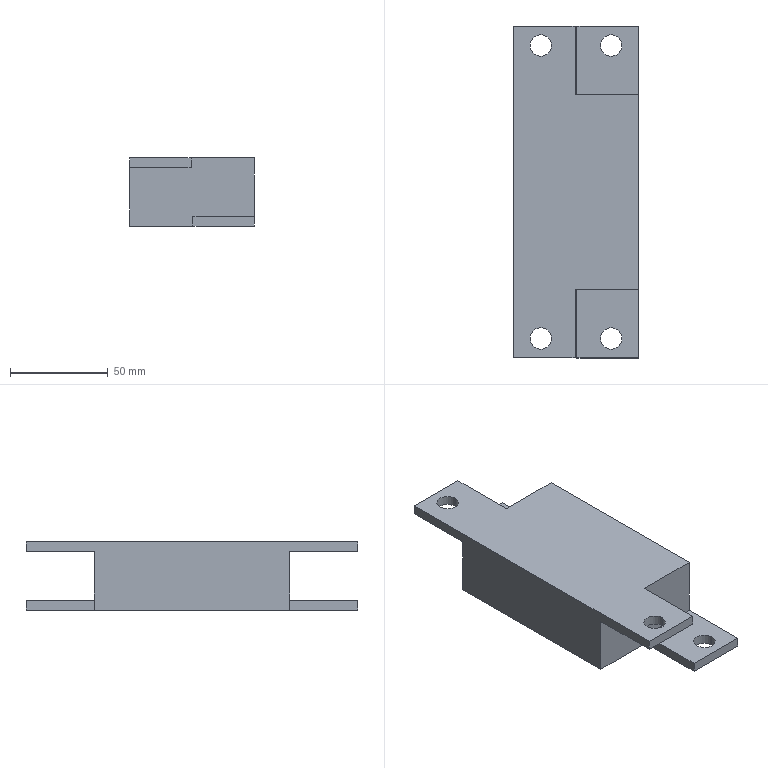Part | SolidWorks | features ICE 3, Extrusion 1 | 1 solid | 26 faces | box 64 x 170 x 35 mm | volume 244149 mm3 | plane 18 | cylinder 8 | commonest cylinder face diameters 11 x8
STEP:
#1=CARTESIAN_POINT('',(12.5,-75.,0.));
#2=VERTEX_POINT('',#1);
#3=CARTESIAN_POINT('',(23.5,-75.,0.));
#4=VERTEX_POINT('',#3);
#5=CARTESIAN_POINT('',(18.,-75.,0.));
#6=DIRECTION('',(0.,0.,1.));
#7=DIRECTION('',(-1.,0.,0.));
#8=AXIS2_PLACEMENT_3D('',#5,#6,#7);
#9=CIRCLE('',#8,5.5);
#10=EDGE_CURVE('',#2,#4,#9,.T.);
#11=ORIENTED_EDGE('',*,*,#10,.F.);
#12=CARTESIAN_POINT('',(12.5,-75.,5.));
#13=VERTEX_POINT('',#12);
#14=CARTESIAN_POINT('',(12.5,-75.,0.));
#15=DIRECTION('',(0.,0.,1.));
#16=VECTOR('',#15,1000.);
#17=LINE('',#14,#16);
#18=EDGE_CURVE('',#2,#13,#17,.T.);
#19=ORIENTED_EDGE('',*,*,#18,.T.);
#20=CARTESIAN_POINT('',(23.5,-75.,5.));
#21=VERTEX_POINT('',#20);
#22=CARTESIAN_POINT('',(18.,-75.,5.));
#23=DIRECTION('',(0.,0.,1.));
#24=DIRECTION('',(1.,0.,0.));
#25=AXIS2_PLACEMENT_3D('',#22,#23,#24);
#26=CIRCLE('',#25,5.5);
#27=EDGE_CURVE('',#13,#21,#26,.T.);
#28=ORIENTED_EDGE('',*,*,#27,.T.);
#29=CARTESIAN_POINT('',(23.5,-75.,0.));
#30=DIRECTION('',(0.,0.,1.));
#31=VECTOR('',#30,1000.);
#32=LINE('',#29,#31);
#33=EDGE_CURVE('',#4,#21,#32,.T.);
#34=ORIENTED_EDGE('',*,*,#33,.F.);
#35=EDGE_LOOP('',(#11,#19,#28,#34));
#36=FACE_OUTER_BOUND('',#35,.T.);
#37=CARTESIAN_POINT('',(18.,-75.,0.));
#38=DIRECTION('',(0.,0.,1.));
#39=DIRECTION('',(1.,0.,0.));
#40=AXIS2_PLACEMENT_3D('',#37,#38,#39);
#41=CYLINDRICAL_SURFACE('',#40,5.5);
#42=ADVANCED_FACE('',(#36),#41,.F.);
#43=CARTESIAN_POINT('',(12.5,75.,0.));
#44=VERTEX_POINT('',#43);
#45=CARTESIAN_POINT('',(23.5,75.,0.));
#46=VERTEX_POINT('',#45);
#47=CARTESIAN_POINT('',(18.,75.,0.));
#48=DIRECTION('',(0.,0.,1.));
#49=DIRECTION('',(1.,0.,0.));
#50=AXIS2_PLACEMENT_3D('',#47,#48,#49);
#51=CIRCLE('',#50,5.5);
#52=EDGE_CURVE('',#44,#46,#51,.T.);
#53=ORIENTED_EDGE('',*,*,#52,.F.);
#54=CARTESIAN_POINT('',(12.5,75.,5.));
#55=VERTEX_POINT('',#54);
#56=CARTESIAN_POINT('',(12.5,75.,0.));
#57=DIRECTION('',(0.,0.,1.));
#58=VECTOR('',#57,1000.);
#59=LINE('',#56,#58);
#60=EDGE_CURVE('',#44,#55,#59,.T.);
#61=ORIENTED_EDGE('',*,*,#60,.T.);
#62=CARTESIAN_POINT('',(23.5,75.,5.));
#63=VERTEX_POINT('',#62);
#64=CARTESIAN_POINT('',(18.,75.,5.));
#65=DIRECTION('',(0.,0.,-1.));
#66=DIRECTION('',(-1.,0.,0.));
#67=AXIS2_PLACEMENT_3D('',#64,#65,#66);
#68=CIRCLE('',#67,5.5);
#69=EDGE_CURVE('',#63,#55,#68,.T.);
#70=ORIENTED_EDGE('',*,*,#69,.F.);
#71=CARTESIAN_POINT('',(23.5,75.,0.));
#72=DIRECTION('',(0.,0.,1.));
#73=VECTOR('',#72,1000.);
#74=LINE('',#71,#73);
#75=EDGE_CURVE('',#46,#63,#74,.T.);
#76=ORIENTED_EDGE('',*,*,#75,.F.);
#77=EDGE_LOOP('',(#53,#61,#70,#76));
#78=FACE_OUTER_BOUND('',#77,.T.);
#79=CARTESIAN_POINT('',(18.,75.,0.));
#80=DIRECTION('',(0.,0.,1.));
#81=DIRECTION('',(1.,0.,0.));
#82=AXIS2_PLACEMENT_3D('',#79,#80,#81);
#83=CYLINDRICAL_SURFACE('',#82,5.5);
#84=ADVANCED_FACE('',(#78),#83,.F.);
#85=CARTESIAN_POINT('',(-23.5,75.,30.));
#86=VERTEX_POINT('',#85);
#87=CARTESIAN_POINT('',(-12.5,75.,30.));
#88=VERTEX_POINT('',#87);
#89=CARTESIAN_POINT('',(-18.,75.,30.));
#90=DIRECTION('',(0.,0.,1.));
#91=DIRECTION('',(1.,0.,0.));
#92=AXIS2_PLACEMENT_3D('',#89,#90,#91);
#93=CIRCLE('',#92,5.5);
#94=EDGE_CURVE('',#86,#88,#93,.T.);
#95=ORIENTED_EDGE('',*,*,#94,.F.);
#96=CARTESIAN_POINT('',(-23.5,75.,35.));
#97=VERTEX_POINT('',#96);
#98=CARTESIAN_POINT('',(-23.5,75.,0.));
#99=DIRECTION('',(0.,0.,1.));
#100=VECTOR('',#99,1000.);
#101=LINE('',#98,#100);
#102=EDGE_CURVE('',#86,#97,#101,.T.);
#103=ORIENTED_EDGE('',*,*,#102,.T.);
#104=CARTESIAN_POINT('',(-12.5,75.,35.));
#105=VERTEX_POINT('',#104);
#106=CARTESIAN_POINT('',(-18.,75.,35.));
#107=DIRECTION('',(0.,0.,1.));
#108=DIRECTION('',(1.,0.,0.));
#109=AXIS2_PLACEMENT_3D('',#106,#107,#108);
#110=CIRCLE('',#109,5.5);
#111=EDGE_CURVE('',#97,#105,#110,.T.);
#112=ORIENTED_EDGE('',*,*,#111,.T.);
#113=CARTESIAN_POINT('',(-12.5,75.,0.));
#114=DIRECTION('',(0.,0.,1.));
#115=VECTOR('',#114,1000.);
#116=LINE('',#113,#115);
#117=EDGE_CURVE('',#88,#105,#116,.T.);
#118=ORIENTED_EDGE('',*,*,#117,.F.);
#119=EDGE_LOOP('',(#95,#103,#112,#118));
#120=FACE_OUTER_BOUND('',#119,.T.);
#121=CARTESIAN_POINT('',(-18.,75.,0.));
#122=DIRECTION('',(0.,0.,1.));
#123=DIRECTION('',(1.,0.,0.));
#124=AXIS2_PLACEMENT_3D('',#121,#122,#123);
#125=CYLINDRICAL_SURFACE('',#124,5.5);
#126=ADVANCED_FACE('',(#120),#125,.F.);
#127=CARTESIAN_POINT('',(-12.5,-75.,30.));
#128=VERTEX_POINT('',#127);
#129=CARTESIAN_POINT('',(-23.5,-75.,30.));
#130=VERTEX_POINT('',#129);
#131=CARTESIAN_POINT('',(-18.,-75.,30.));
#132=DIRECTION('',(0.,0.,-1.));
#133=DIRECTION('',(-1.,0.,0.));
#134=AXIS2_PLACEMENT_3D('',#131,#132,#133);
#135=CIRCLE('',#134,5.5);
#136=EDGE_CURVE('',#128,#130,#135,.T.);
#137=ORIENTED_EDGE('',*,*,#136,.T.);
#138=CARTESIAN_POINT('',(-23.5,-75.,35.));
#139=VERTEX_POINT('',#138);
#140=CARTESIAN_POINT('',(-23.5,-75.,0.));
#141=DIRECTION('',(0.,0.,1.));
#142=VECTOR('',#141,1000.);
#143=LINE('',#140,#142);
#144=EDGE_CURVE('',#130,#139,#143,.T.);
#145=ORIENTED_EDGE('',*,*,#144,.T.);
#146=CARTESIAN_POINT('',(-12.5,-75.,35.));
#147=VERTEX_POINT('',#146);
#148=CARTESIAN_POINT('',(-18.,-75.,35.));
#149=DIRECTION('',(0.,0.,1.));
#150=DIRECTION('',(1.,0.,0.));
#151=AXIS2_PLACEMENT_3D('',#148,#149,#150);
#152=CIRCLE('',#151,5.5);
#153=EDGE_CURVE('',#139,#147,#152,.T.);
#154=ORIENTED_EDGE('',*,*,#153,.T.);
#155=CARTESIAN_POINT('',(-12.5,-75.,0.));
#156=DIRECTION('',(0.,0.,1.));
#157=VECTOR('',#156,1000.);
#158=LINE('',#155,#157);
#159=EDGE_CURVE('',#128,#147,#158,.T.);
#160=ORIENTED_EDGE('',*,*,#159,.F.);
#161=EDGE_LOOP('',(#137,#145,#154,#160));
#162=FACE_OUTER_BOUND('',#161,.T.);
#163=CARTESIAN_POINT('',(-18.,-75.,0.));
#164=DIRECTION('',(0.,0.,1.));
#165=DIRECTION('',(1.,0.,0.));
#166=AXIS2_PLACEMENT_3D('',#163,#164,#165);
#167=CYLINDRICAL_SURFACE('',#166,5.5);
#168=ADVANCED_FACE('',(#162),#167,.F.);
#169=CARTESIAN_POINT('',(32.,85.,0.));
#170=VERTEX_POINT('',#169);
#171=CARTESIAN_POINT('',(0.5,85.,0.));
#172=VERTEX_POINT('',#171);
#173=CARTESIAN_POINT('',(-32.,85.,0.));
#174=DIRECTION('',(-1.,0.,0.));
#175=VECTOR('',#174,1000.);
#176=LINE('',#173,#175);
#177=EDGE_CURVE('',#170,#172,#176,.T.);
#178=ORIENTED_EDGE('',*,*,#177,.T.);
#179=CARTESIAN_POINT('',(0.5,85.,5.));
#180=VERTEX_POINT('',#179);
#181=CARTESIAN_POINT('',(0.5,85.,30.));
#182=DIRECTION('',(0.,0.,-1.));
#183=VECTOR('',#182,1000.);
#184=LINE('',#181,#183);
#185=EDGE_CURVE('',#180,#172,#184,.T.);
#186=ORIENTED_EDGE('',*,*,#185,.F.);
#187=CARTESIAN_POINT('',(32.,85.,5.));
#188=VERTEX_POINT('',#187);
#189=CARTESIAN_POINT('',(32.,85.,5.));
#190=DIRECTION('',(-1.,0.,0.));
#191=VECTOR('',#190,1000.);
#192=LINE('',#189,#191);
#193=EDGE_CURVE('',#188,#180,#192,.T.);
#194=ORIENTED_EDGE('',*,*,#193,.F.);
#195=CARTESIAN_POINT('',(32.,85.,35.));
#196=DIRECTION('',(0.,0.,-1.));
#197=VECTOR('',#196,1000.);
#198=LINE('',#195,#197);
#199=EDGE_CURVE('',#188,#170,#198,.T.);
#200=ORIENTED_EDGE('',*,*,#199,.T.);
#201=EDGE_LOOP('',(#178,#186,#194,#200));
#202=FACE_OUTER_BOUND('',#201,.T.);
#203=CARTESIAN_POINT('',(-32.,85.,35.));
#204=DIRECTION('',(0.,-1.,0.));
#205=DIRECTION('',(0.,0.,-1.));
#206=AXIS2_PLACEMENT_3D('',#203,#204,#205);
#207=PLANE('',#206);
#208=ADVANCED_FACE('',(#202),#207,.F.);
#209=CARTESIAN_POINT('',(-0.5,-85.,30.));
#210=VERTEX_POINT('',#209);
#211=CARTESIAN_POINT('',(-32.,-85.,30.));
#212=VERTEX_POINT('',#211);
#213=CARTESIAN_POINT('',(-32.,-85.,30.));
#214=DIRECTION('',(-1.,0.,0.));
#215=VECTOR('',#214,1000.);
#216=LINE('',#213,#215);
#217=EDGE_CURVE('',#210,#212,#216,.T.);
#218=ORIENTED_EDGE('',*,*,#217,.F.);
#219=CARTESIAN_POINT('',(-0.5,-85.,35.));
#220=VERTEX_POINT('',#219);
#221=CARTESIAN_POINT('',(-0.5,-85.,5.));
#222=DIRECTION('',(0.,0.,1.));
#223=VECTOR('',#222,1000.);
#224=LINE('',#221,#223);
#225=EDGE_CURVE('',#210,#220,#224,.T.);
#226=ORIENTED_EDGE('',*,*,#225,.T.);
#227=CARTESIAN_POINT('',(-32.,-85.,35.));
#228=VERTEX_POINT('',#227);
#229=CARTESIAN_POINT('',(-32.,-85.,35.));
#230=DIRECTION('',(1.,0.,0.));
#231=VECTOR('',#230,1000.);
#232=LINE('',#229,#231);
#233=EDGE_CURVE('',#228,#220,#232,.T.);
#234=ORIENTED_EDGE('',*,*,#233,.F.);
#235=CARTESIAN_POINT('',(-32.,-85.,35.));
#236=DIRECTION('',(0.,0.,-1.));
#237=VECTOR('',#236,1000.);
#238=LINE('',#235,#237);
#239=EDGE_CURVE('',#228,#212,#238,.T.);
#240=ORIENTED_EDGE('',*,*,#239,.T.);
#241=EDGE_LOOP('',(#218,#226,#234,#240));
#242=FACE_OUTER_BOUND('',#241,.T.);
#243=CARTESIAN_POINT('',(-32.,-85.,35.));
#244=DIRECTION('',(0.,1.,0.));
#245=DIRECTION('',(0.,0.,1.));
#246=AXIS2_PLACEMENT_3D('',#243,#244,#245);
#247=PLANE('',#246);
#248=ADVANCED_FACE('',(#242),#247,.F.);
#249=CARTESIAN_POINT('',(-0.5,-50.,30.));
#250=VERTEX_POINT('',#249);
#251=CARTESIAN_POINT('',(-0.5,-85.,30.));
#252=DIRECTION('',(0.,-1.,0.));
#253=VECTOR('',#252,1000.);
#254=LINE('',#251,#253);
#255=EDGE_CURVE('',#250,#210,#254,.T.);
#256=ORIENTED_EDGE('',*,*,#255,.F.);
#257=CARTESIAN_POINT('',(-0.5,-50.,35.));
#258=VERTEX_POINT('',#257);
#259=CARTESIAN_POINT('',(-0.5,-50.,5.));
#260=DIRECTION('',(0.,0.,1.));
#261=VECTOR('',#260,1000.);
#262=LINE('',#259,#261);
#263=EDGE_CURVE('',#250,#258,#262,.T.);
#264=ORIENTED_EDGE('',*,*,#263,.T.);
#265=CARTESIAN_POINT('',(-0.5,-85.,35.));
#266=DIRECTION('',(0.,-1.,0.));
#267=VECTOR('',#266,1000.);
#268=LINE('',#265,#267);
#269=EDGE_CURVE('',#258,#220,#268,.T.);
#270=ORIENTED_EDGE('',*,*,#269,.T.);
#271=ORIENTED_EDGE('',*,*,#225,.F.);
#272=EDGE_LOOP('',(#256,#264,#270,#271));
#273=FACE_OUTER_BOUND('',#272,.T.);
#274=CARTESIAN_POINT('',(-0.5,-85.,5.));
#275=DIRECTION('',(-1.,0.,0.));
#276=DIRECTION('',(0.,0.,1.));
#277=AXIS2_PLACEMENT_3D('',#274,#275,#276);
#278=PLANE('',#277);
#279=ADVANCED_FACE('',(#273),#278,.F.);
#280=CARTESIAN_POINT('',(32.,50.,5.));
#281=VERTEX_POINT('',#280);
#282=CARTESIAN_POINT('',(32.,85.,5.));
#283=DIRECTION('',(0.,1.,0.));
#284=VECTOR('',#283,1000.);
#285=LINE('',#282,#284);
#286=EDGE_CURVE('',#281,#188,#285,.T.);
#287=ORIENTED_EDGE('',*,*,#286,.F.);
#288=CARTESIAN_POINT('',(32.,50.,35.));
#289=VERTEX_POINT('',#288);
#290=CARTESIAN_POINT('',(32.,50.,5.));
#291=DIRECTION('',(0.,0.,1.));
#292=VECTOR('',#291,1000.);
#293=LINE('',#290,#292);
#294=EDGE_CURVE('',#281,#289,#293,.T.);
#295=ORIENTED_EDGE('',*,*,#294,.T.);
#296=CARTESIAN_POINT('',(32.,-50.,35.));
#297=VERTEX_POINT('',#296);
#298=CARTESIAN_POINT('',(32.,85.,35.));
#299=DIRECTION('',(0.,1.,0.));
#300=VECTOR('',#299,1000.);
#301=LINE('',#298,#300);
#302=EDGE_CURVE('',#297,#289,#301,.T.);
#303=ORIENTED_EDGE('',*,*,#302,.F.);
#304=CARTESIAN_POINT('',(32.,-50.,5.));
#305=VERTEX_POINT('',#304);
#306=CARTESIAN_POINT('',(32.,-50.,5.));
#307=DIRECTION('',(0.,0.,1.));
#308=VECTOR('',#307,1000.);
#309=LINE('',#306,#308);
#310=EDGE_CURVE('',#305,#297,#309,.T.);
#311=ORIENTED_EDGE('',*,*,#310,.F.);
#312=CARTESIAN_POINT('',(32.,-85.,5.));
#313=VERTEX_POINT('',#312);
#314=CARTESIAN_POINT('',(32.,-85.,5.));
#315=DIRECTION('',(0.,1.,0.));
#316=VECTOR('',#315,1000.);
#317=LINE('',#314,#316);
#318=EDGE_CURVE('',#313,#305,#317,.T.);
#319=ORIENTED_EDGE('',*,*,#318,.F.);
#320=CARTESIAN_POINT('',(32.,-85.,0.));
#321=VERTEX_POINT('',#320);
#322=CARTESIAN_POINT('',(32.,-85.,35.));
#323=DIRECTION('',(0.,0.,-1.));
#324=VECTOR('',#323,1000.);
#325=LINE('',#322,#324);
#326=EDGE_CURVE('',#313,#321,#325,.T.);
#327=ORIENTED_EDGE('',*,*,#326,.T.);
#328=CARTESIAN_POINT('',(32.,85.,0.));
#329=DIRECTION('',(0.,1.,0.));
#330=VECTOR('',#329,1000.);
#331=LINE('',#328,#330);
#332=EDGE_CURVE('',#321,#170,#331,.T.);
#333=ORIENTED_EDGE('',*,*,#332,.T.);
#334=ORIENTED_EDGE('',*,*,#199,.F.);
#335=EDGE_LOOP('',(#287,#295,#303,#311,#319,#327,#333,#334));
#336=FACE_OUTER_BOUND('',#335,.T.);
#337=CARTESIAN_POINT('',(32.,85.,35.));
#338=DIRECTION('',(-1.,0.,0.));
#339=DIRECTION('',(0.,-1.,0.));
#340=AXIS2_PLACEMENT_3D('',#337,#338,#339);
#341=PLANE('',#340);
#342=ADVANCED_FACE('',(#336),#341,.F.);
#343=CARTESIAN_POINT('',(-0.5,85.,30.));
#344=VERTEX_POINT('',#343);
#345=CARTESIAN_POINT('',(-0.5,85.,35.));
#346=VERTEX_POINT('',#345);
#347=CARTESIAN_POINT('',(-0.5,85.,5.));
#348=DIRECTION('',(0.,0.,1.));
#349=VECTOR('',#348,1000.);
#350=LINE('',#347,#349);
#351=EDGE_CURVE('',#344,#346,#350,.T.);
#352=ORIENTED_EDGE('',*,*,#351,.F.);
#353=CARTESIAN_POINT('',(-32.,85.,30.));
#354=VERTEX_POINT('',#353);
#355=CARTESIAN_POINT('',(-32.,85.,30.));
#356=DIRECTION('',(1.,0.,0.));
#357=VECTOR('',#356,1000.);
#358=LINE('',#355,#357);
#359=EDGE_CURVE('',#354,#344,#358,.T.);
#360=ORIENTED_EDGE('',*,*,#359,.F.);
#361=CARTESIAN_POINT('',(-32.,85.,35.));
#362=VERTEX_POINT('',#361);
#363=CARTESIAN_POINT('',(-32.,85.,35.));
#364=DIRECTION('',(0.,0.,-1.));
#365=VECTOR('',#364,1000.);
#366=LINE('',#363,#365);
#367=EDGE_CURVE('',#362,#354,#366,.T.);
#368=ORIENTED_EDGE('',*,*,#367,.F.);
#369=CARTESIAN_POINT('',(-32.,85.,35.));
#370=DIRECTION('',(-1.,0.,0.));
#371=VECTOR('',#370,1000.);
#372=LINE('',#369,#371);
#373=EDGE_CURVE('',#346,#362,#372,.T.);
#374=ORIENTED_EDGE('',*,*,#373,.F.);
#375=EDGE_LOOP('',(#352,#360,#368,#374));
#376=FACE_OUTER_BOUND('',#375,.T.);
#377=CARTESIAN_POINT('',(-32.,85.,35.));
#378=DIRECTION('',(0.,-1.,0.));
#379=DIRECTION('',(0.,0.,-1.));
#380=AXIS2_PLACEMENT_3D('',#377,#378,#379);
#381=PLANE('',#380);
#382=ADVANCED_FACE('',(#376),#381,.F.);
#383=CARTESIAN_POINT('',(-32.,50.,30.));
#384=VERTEX_POINT('',#383);
#385=CARTESIAN_POINT('',(-32.,85.,30.));
#386=DIRECTION('',(0.,1.,0.));
#387=VECTOR('',#386,1000.);
#388=LINE('',#385,#387);
#389=EDGE_CURVE('',#384,#354,#388,.T.);
#390=ORIENTED_EDGE('',*,*,#389,.F.);
#391=CARTESIAN_POINT('',(-32.,50.,0.));
#392=VERTEX_POINT('',#391);
#393=CARTESIAN_POINT('',(-32.,50.,30.));
#394=DIRECTION('',(0.,0.,-1.));
#395=VECTOR('',#394,1000.);
#396=LINE('',#393,#395);
#397=EDGE_CURVE('',#384,#392,#396,.T.);
#398=ORIENTED_EDGE('',*,*,#397,.T.);
#399=CARTESIAN_POINT('',(-32.,-50.,0.));
#400=VERTEX_POINT('',#399);
#401=CARTESIAN_POINT('',(-32.,85.,0.));
#402=DIRECTION('',(0.,-1.,0.));
#403=VECTOR('',#402,1000.);
#404=LINE('',#401,#403);
#405=EDGE_CURVE('',#392,#400,#404,.T.);
#406=ORIENTED_EDGE('',*,*,#405,.T.);
#407=CARTESIAN_POINT('',(-32.,-50.,30.));
#408=VERTEX_POINT('',#407);
#409=CARTESIAN_POINT('',(-32.,-50.,30.));
#410=DIRECTION('',(0.,0.,-1.));
#411=VECTOR('',#410,1000.);
#412=LINE('',#409,#411);
#413=EDGE_CURVE('',#408,#400,#412,.T.);
#414=ORIENTED_EDGE('',*,*,#413,.F.);
#415=CARTESIAN_POINT('',(-32.,-85.,30.));
#416=DIRECTION('',(0.,1.,0.));
#417=VECTOR('',#416,1000.);
#418=LINE('',#415,#417);
#419=EDGE_CURVE('',#212,#408,#418,.T.);
#420=ORIENTED_EDGE('',*,*,#419,.F.);
#421=ORIENTED_EDGE('',*,*,#239,.F.);
#422=CARTESIAN_POINT('',(-32.,85.,35.));
#423=DIRECTION('',(0.,-1.,0.));
#424=VECTOR('',#423,1000.);
#425=LINE('',#422,#424);
#426=EDGE_CURVE('',#362,#228,#425,.T.);
#427=ORIENTED_EDGE('',*,*,#426,.F.);
#428=ORIENTED_EDGE('',*,*,#367,.T.);
#429=EDGE_LOOP('',(#390,#398,#406,#414,#420,#421,#427,#428));
#430=FACE_OUTER_BOUND('',#429,.T.);
#431=CARTESIAN_POINT('',(-32.,85.,35.));
#432=DIRECTION('',(1.,0.,0.));
#433=DIRECTION('',(0.,1.,0.));
#434=AXIS2_PLACEMENT_3D('',#431,#432,#433);
#435=PLANE('',#434);
#436=ADVANCED_FACE('',(#430),#435,.F.);
#437=CARTESIAN_POINT('',(0.5,-85.,5.));
#438=VERTEX_POINT('',#437);
#439=CARTESIAN_POINT('',(32.,-85.,5.));
#440=DIRECTION('',(1.,0.,0.));
#441=VECTOR('',#440,1000.);
#442=LINE('',#439,#441);
#443=EDGE_CURVE('',#438,#313,#442,.T.);
#444=ORIENTED_EDGE('',*,*,#443,.F.);
#445=CARTESIAN_POINT('',(0.5,-85.,0.));
#446=VERTEX_POINT('',#445);
#447=CARTESIAN_POINT('',(0.5,-85.,30.));
#448=DIRECTION('',(0.,0.,-1.));
#449=VECTOR('',#448,1000.);
#450=LINE('',#447,#449);
#451=EDGE_CURVE('',#438,#446,#450,.T.);
#452=ORIENTED_EDGE('',*,*,#451,.T.);
#453=CARTESIAN_POINT('',(-32.,-85.,0.));
#454=DIRECTION('',(1.,0.,0.));
#455=VECTOR('',#454,1000.);
#456=LINE('',#453,#455);
#457=EDGE_CURVE('',#446,#321,#456,.T.);
#458=ORIENTED_EDGE('',*,*,#457,.T.);
#459=ORIENTED_EDGE('',*,*,#326,.F.);
#460=EDGE_LOOP('',(#444,#452,#458,#459));
#461=FACE_OUTER_BOUND('',#460,.T.);
#462=CARTESIAN_POINT('',(-32.,-85.,35.));
#463=DIRECTION('',(0.,1.,0.));
#464=DIRECTION('',(0.,0.,1.));
#465=AXIS2_PLACEMENT_3D('',#462,#463,#464);
#466=PLANE('',#465);
#467=ADVANCED_FACE('',(#461),#466,.F.);
#468=CARTESIAN_POINT('',(-18.,-75.,35.));
#469=DIRECTION('',(0.,0.,1.));
#470=DIRECTION('',(1.,0.,0.));
#471=AXIS2_PLACEMENT_3D('',#468,#469,#470);
#472=CIRCLE('',#471,5.5);
#473=EDGE_CURVE('',#147,#139,#472,.T.);
#474=ORIENTED_EDGE('',*,*,#473,.F.);
#475=ORIENTED_EDGE('',*,*,#153,.F.);
#476=EDGE_LOOP('',(#474,#475));
#477=FACE_BOUND('',#476,.T.);
#478=CARTESIAN_POINT('',(-18.,75.,35.));
#479=DIRECTION('',(0.,0.,1.));
#480=DIRECTION('',(1.,0.,0.));
#481=AXIS2_PLACEMENT_3D('',#478,#479,#480);
#482=CIRCLE('',#481,5.5);
#483=EDGE_CURVE('',#105,#97,#482,.T.);
#484=ORIENTED_EDGE('',*,*,#483,.F.);
#485=ORIENTED_EDGE('',*,*,#111,.F.);
#486=EDGE_LOOP('',(#484,#485));
#487=FACE_BOUND('',#486,.T.);
#488=CARTESIAN_POINT('',(-0.5,50.,35.));
#489=VERTEX_POINT('',#488);
#490=CARTESIAN_POINT('',(32.,50.,35.));
#491=DIRECTION('',(1.,0.,0.));
#492=VECTOR('',#491,1000.);
#493=LINE('',#490,#492);
#494=EDGE_CURVE('',#489,#289,#493,.T.);
#495=ORIENTED_EDGE('',*,*,#494,.F.);
#496=CARTESIAN_POINT('',(-0.5,85.,35.));
#497=DIRECTION('',(0.,-1.,0.));
#498=VECTOR('',#497,1000.);
#499=LINE('',#496,#498);
#500=EDGE_CURVE('',#346,#489,#499,.T.);
#501=ORIENTED_EDGE('',*,*,#500,.F.);
#502=ORIENTED_EDGE('',*,*,#373,.T.);
#503=ORIENTED_EDGE('',*,*,#426,.T.);
#504=ORIENTED_EDGE('',*,*,#233,.T.);
#505=ORIENTED_EDGE('',*,*,#269,.F.);
#506=CARTESIAN_POINT('',(32.,-50.,35.));
#507=DIRECTION('',(-1.,0.,0.));
#508=VECTOR('',#507,1000.);
#509=LINE('',#506,#508);
#510=EDGE_CURVE('',#297,#258,#509,.T.);
#511=ORIENTED_EDGE('',*,*,#510,.F.);
#512=ORIENTED_EDGE('',*,*,#302,.T.);
#513=EDGE_LOOP('',(#495,#501,#502,#503,#504,#505,#511,#512));
#514=FACE_OUTER_BOUND('',#513,.T.);
#515=CARTESIAN_POINT('',(0.,0.,35.));
#516=DIRECTION('',(0.,0.,1.));
#517=DIRECTION('',(1.,0.,0.));
#518=AXIS2_PLACEMENT_3D('',#515,#516,#517);
#519=PLANE('',#518);
#520=ADVANCED_FACE('',(#477,#487,#514),#519,.T.);
#521=CARTESIAN_POINT('',(18.,-75.,0.));
#522=DIRECTION('',(0.,0.,1.));
#523=DIRECTION('',(-1.,0.,0.));
#524=AXIS2_PLACEMENT_3D('',#521,#522,#523);
#525=CIRCLE('',#524,5.5);
#526=EDGE_CURVE('',#4,#2,#525,.T.);
#527=ORIENTED_EDGE('',*,*,#526,.T.);
#528=ORIENTED_EDGE('',*,*,#10,.T.);
#529=EDGE_LOOP('',(#527,#528));
#530=FACE_BOUND('',#529,.T.);
#531=CARTESIAN_POINT('',(18.,75.,0.));
#532=DIRECTION('',(0.,0.,1.));
#533=DIRECTION('',(1.,0.,0.));
#534=AXIS2_PLACEMENT_3D('',#531,#532,#533);
#535=CIRCLE('',#534,5.5);
#536=EDGE_CURVE('',#46,#44,#535,.T.);
#537=ORIENTED_EDGE('',*,*,#536,.T.);
#538=ORIENTED_EDGE('',*,*,#52,.T.);
#539=EDGE_LOOP('',(#537,#538));
#540=FACE_BOUND('',#539,.T.);
#541=ORIENTED_EDGE('',*,*,#405,.F.);
#542=CARTESIAN_POINT('',(0.5,50.,0.));
#543=VERTEX_POINT('',#542);
#544=CARTESIAN_POINT('',(-32.,50.,0.));
#545=DIRECTION('',(-1.,0.,0.));
#546=VECTOR('',#545,1000.);
#547=LINE('',#544,#546);
#548=EDGE_CURVE('',#543,#392,#547,.T.);
#549=ORIENTED_EDGE('',*,*,#548,.F.);
#550=CARTESIAN_POINT('',(0.5,85.,0.));
#551=DIRECTION('',(0.,-1.,0.));
#552=VECTOR('',#551,1000.);
#553=LINE('',#550,#552);
#554=EDGE_CURVE('',#172,#543,#553,.T.);
#555=ORIENTED_EDGE('',*,*,#554,.F.);
#556=ORIENTED_EDGE('',*,*,#177,.F.);
#557=ORIENTED_EDGE('',*,*,#332,.F.);
#558=ORIENTED_EDGE('',*,*,#457,.F.);
#559=CARTESIAN_POINT('',(0.5,-50.,0.));
#560=VERTEX_POINT('',#559);
#561=CARTESIAN_POINT('',(0.5,-85.,0.));
#562=DIRECTION('',(0.,-1.,0.));
#563=VECTOR('',#562,1000.);
#564=LINE('',#561,#563);
#565=EDGE_CURVE('',#560,#446,#564,.T.);
#566=ORIENTED_EDGE('',*,*,#565,.F.);
#567=CARTESIAN_POINT('',(-32.,-50.,0.));
#568=DIRECTION('',(1.,0.,0.));
#569=VECTOR('',#568,1000.);
#570=LINE('',#567,#569);
#571=EDGE_CURVE('',#400,#560,#570,.T.);
#572=ORIENTED_EDGE('',*,*,#571,.F.);
#573=EDGE_LOOP('',(#541,#549,#555,#556,#557,#558,#566,#572));
#574=FACE_OUTER_BOUND('',#573,.T.);
#575=CARTESIAN_POINT('',(0.,0.,0.));
#576=DIRECTION('',(0.,0.,1.));
#577=DIRECTION('',(1.,0.,0.));
#578=AXIS2_PLACEMENT_3D('',#575,#576,#577);
#579=PLANE('',#578);
#580=ADVANCED_FACE('',(#530,#540,#574),#579,.F.);
#581=ORIENTED_EDGE('',*,*,#263,.F.);
#582=CARTESIAN_POINT('',(-32.,-50.,30.));
#583=DIRECTION('',(1.,0.,0.));
#584=VECTOR('',#583,1000.);
#585=LINE('',#582,#584);
#586=EDGE_CURVE('',#408,#250,#585,.T.);
#587=ORIENTED_EDGE('',*,*,#586,.F.);
#588=ORIENTED_EDGE('',*,*,#413,.T.);
#589=ORIENTED_EDGE('',*,*,#571,.T.);
#590=CARTESIAN_POINT('',(0.5,-50.,5.));
#591=VERTEX_POINT('',#590);
#592=CARTESIAN_POINT('',(0.5,-50.,30.));
#593=DIRECTION('',(0.,0.,-1.));
#594=VECTOR('',#593,1000.);
#595=LINE('',#592,#594);
#596=EDGE_CURVE('',#591,#560,#595,.T.);
#597=ORIENTED_EDGE('',*,*,#596,.F.);
#598=CARTESIAN_POINT('',(32.,-50.,5.));
#599=DIRECTION('',(-1.,0.,0.));
#600=VECTOR('',#599,1000.);
#601=LINE('',#598,#600);
#602=EDGE_CURVE('',#305,#591,#601,.T.);
#603=ORIENTED_EDGE('',*,*,#602,.F.);
#604=ORIENTED_EDGE('',*,*,#310,.T.);
#605=ORIENTED_EDGE('',*,*,#510,.T.);
#606=EDGE_LOOP('',(#581,#587,#588,#589,#597,#603,#604,#605));
#607=FACE_OUTER_BOUND('',#606,.T.);
#608=CARTESIAN_POINT('',(32.,-50.,5.));
#609=DIRECTION('',(0.,1.,0.));
#610=DIRECTION('',(-1.,0.,0.));
#611=AXIS2_PLACEMENT_3D('',#608,#609,#610);
#612=PLANE('',#611);
#613=ADVANCED_FACE('',(#607),#612,.F.);
#614=CARTESIAN_POINT('',(18.,-75.,5.));
#615=DIRECTION('',(0.,0.,1.));
#616=DIRECTION('',(1.,0.,0.));
#617=AXIS2_PLACEMENT_3D('',#614,#615,#616);
#618=CIRCLE('',#617,5.5);
#619=EDGE_CURVE('',#21,#13,#618,.T.);
#620=ORIENTED_EDGE('',*,*,#619,.F.);
#621=ORIENTED_EDGE('',*,*,#27,.F.);
#622=EDGE_LOOP('',(#620,#621));
#623=FACE_BOUND('',#622,.T.);
#624=CARTESIAN_POINT('',(0.5,0.,5.));
#625=DIRECTION('',(0.,1.,0.));
#626=VECTOR('',#625,1000.);
#627=LINE('',#624,#626);
#628=EDGE_CURVE('',#438,#591,#627,.T.);
#629=ORIENTED_EDGE('',*,*,#628,.F.);
#630=ORIENTED_EDGE('',*,*,#443,.T.);
#631=ORIENTED_EDGE('',*,*,#318,.T.);
#632=ORIENTED_EDGE('',*,*,#602,.T.);
#633=EDGE_LOOP('',(#629,#630,#631,#632));
#634=FACE_OUTER_BOUND('',#633,.T.);
#635=CARTESIAN_POINT('',(0.,0.,5.));
#636=DIRECTION('',(0.,0.,1.));
#637=DIRECTION('',(1.,0.,0.));
#638=AXIS2_PLACEMENT_3D('',#635,#636,#637);
#639=PLANE('',#638);
#640=ADVANCED_FACE('',(#623,#634),#639,.T.);
#641=CARTESIAN_POINT('',(0.5,50.,5.));
#642=VERTEX_POINT('',#641);
#643=CARTESIAN_POINT('',(32.,50.,5.));
#644=DIRECTION('',(1.,0.,0.));
#645=VECTOR('',#644,1000.);
#646=LINE('',#643,#645);
#647=EDGE_CURVE('',#642,#281,#646,.T.);
#648=ORIENTED_EDGE('',*,*,#647,.F.);
#649=CARTESIAN_POINT('',(0.5,50.,30.));
#650=DIRECTION('',(0.,0.,-1.));
#651=VECTOR('',#650,1000.);
#652=LINE('',#649,#651);
#653=EDGE_CURVE('',#642,#543,#652,.T.);
#654=ORIENTED_EDGE('',*,*,#653,.T.);
#655=ORIENTED_EDGE('',*,*,#548,.T.);
#656=ORIENTED_EDGE('',*,*,#397,.F.);
#657=CARTESIAN_POINT('',(-0.5,50.,30.));
#658=VERTEX_POINT('',#657);
#659=CARTESIAN_POINT('',(-32.,50.,30.));
#660=DIRECTION('',(-1.,0.,0.));
#661=VECTOR('',#660,1000.);
#662=LINE('',#659,#661);
#663=EDGE_CURVE('',#658,#384,#662,.T.);
#664=ORIENTED_EDGE('',*,*,#663,.F.);
#665=CARTESIAN_POINT('',(-0.5,50.,5.));
#666=DIRECTION('',(0.,0.,1.));
#667=VECTOR('',#666,1000.);
#668=LINE('',#665,#667);
#669=EDGE_CURVE('',#658,#489,#668,.T.);
#670=ORIENTED_EDGE('',*,*,#669,.T.);
#671=ORIENTED_EDGE('',*,*,#494,.T.);
#672=ORIENTED_EDGE('',*,*,#294,.F.);
#673=EDGE_LOOP('',(#648,#654,#655,#656,#664,#670,#671,#672));
#674=FACE_OUTER_BOUND('',#673,.T.);
#675=CARTESIAN_POINT('',(32.,50.,5.));
#676=DIRECTION('',(0.,-1.,0.));
#677=DIRECTION('',(1.,0.,0.));
#678=AXIS2_PLACEMENT_3D('',#675,#676,#677);
#679=PLANE('',#678);
#680=ADVANCED_FACE('',(#674),#679,.F.);
#681=ORIENTED_EDGE('',*,*,#669,.F.);
#682=CARTESIAN_POINT('',(-0.5,85.,30.));
#683=DIRECTION('',(0.,1.,0.));
#684=VECTOR('',#683,1000.);
#685=LINE('',#682,#684);
#686=EDGE_CURVE('',#658,#344,#685,.T.);
#687=ORIENTED_EDGE('',*,*,#686,.T.);
#688=ORIENTED_EDGE('',*,*,#351,.T.);
#689=ORIENTED_EDGE('',*,*,#500,.T.);
#690=EDGE_LOOP('',(#681,#687,#688,#689));
#691=FACE_OUTER_BOUND('',#690,.T.);
#692=CARTESIAN_POINT('',(-0.5,85.,5.));
#693=DIRECTION('',(-1.,0.,0.));
#694=DIRECTION('',(0.,-1.,0.));
#695=AXIS2_PLACEMENT_3D('',#692,#693,#694);
#696=PLANE('',#695);
#697=ADVANCED_FACE('',(#691),#696,.F.);
#698=ORIENTED_EDGE('',*,*,#69,.T.);
#699=CARTESIAN_POINT('',(18.,75.,5.));
#700=DIRECTION('',(0.,0.,-1.));
#701=DIRECTION('',(-1.,0.,0.));
#702=AXIS2_PLACEMENT_3D('',#699,#700,#701);
#703=CIRCLE('',#702,5.5);
#704=EDGE_CURVE('',#55,#63,#703,.T.);
#705=ORIENTED_EDGE('',*,*,#704,.T.);
#706=EDGE_LOOP('',(#698,#705));
#707=FACE_BOUND('',#706,.T.);
#708=ORIENTED_EDGE('',*,*,#193,.T.);
#709=CARTESIAN_POINT('',(0.5,0.,5.));
#710=DIRECTION('',(0.,-1.,0.));
#711=VECTOR('',#710,1000.);
#712=LINE('',#709,#711);
#713=EDGE_CURVE('',#180,#642,#712,.T.);
#714=ORIENTED_EDGE('',*,*,#713,.T.);
#715=ORIENTED_EDGE('',*,*,#647,.T.);
#716=ORIENTED_EDGE('',*,*,#286,.T.);
#717=EDGE_LOOP('',(#708,#714,#715,#716));
#718=FACE_OUTER_BOUND('',#717,.T.);
#719=CARTESIAN_POINT('',(0.,0.,5.));
#720=DIRECTION('',(0.,0.,-1.));
#721=DIRECTION('',(-1.,0.,0.));
#722=AXIS2_PLACEMENT_3D('',#719,#720,#721);
#723=PLANE('',#722);
#724=ADVANCED_FACE('',(#707,#718),#723,.F.);
#725=CARTESIAN_POINT('',(-18.,75.,30.));
#726=DIRECTION('',(0.,0.,1.));
#727=DIRECTION('',(1.,0.,0.));
#728=AXIS2_PLACEMENT_3D('',#725,#726,#727);
#729=CIRCLE('',#728,5.5);
#730=EDGE_CURVE('',#88,#86,#729,.T.);
#731=ORIENTED_EDGE('',*,*,#730,.T.);
#732=ORIENTED_EDGE('',*,*,#94,.T.);
#733=EDGE_LOOP('',(#731,#732));
#734=FACE_BOUND('',#733,.T.);
#735=ORIENTED_EDGE('',*,*,#663,.T.);
#736=ORIENTED_EDGE('',*,*,#389,.T.);
#737=ORIENTED_EDGE('',*,*,#359,.T.);
#738=ORIENTED_EDGE('',*,*,#686,.F.);
#739=EDGE_LOOP('',(#735,#736,#737,#738));
#740=FACE_OUTER_BOUND('',#739,.T.);
#741=CARTESIAN_POINT('',(0.,0.,30.));
#742=DIRECTION('',(0.,0.,1.));
#743=DIRECTION('',(1.,0.,0.));
#744=AXIS2_PLACEMENT_3D('',#741,#742,#743);
#745=PLANE('',#744);
#746=ADVANCED_FACE('',(#734,#740),#745,.F.);
#747=ORIENTED_EDGE('',*,*,#185,.T.);
#748=ORIENTED_EDGE('',*,*,#554,.T.);
#749=ORIENTED_EDGE('',*,*,#653,.F.);
#750=ORIENTED_EDGE('',*,*,#713,.F.);
#751=EDGE_LOOP('',(#747,#748,#749,#750));
#752=FACE_OUTER_BOUND('',#751,.T.);
#753=CARTESIAN_POINT('',(0.5,85.,30.));
#754=DIRECTION('',(1.,0.,0.));
#755=DIRECTION('',(0.,1.,0.));
#756=AXIS2_PLACEMENT_3D('',#753,#754,#755);
#757=PLANE('',#756);
#758=ADVANCED_FACE('',(#752),#757,.F.);
#759=ORIENTED_EDGE('',*,*,#136,.F.);
#760=CARTESIAN_POINT('',(-18.,-75.,30.));
#761=DIRECTION('',(0.,0.,-1.));
#762=DIRECTION('',(-1.,0.,0.));
#763=AXIS2_PLACEMENT_3D('',#760,#761,#762);
#764=CIRCLE('',#763,5.5);
#765=EDGE_CURVE('',#130,#128,#764,.T.);
#766=ORIENTED_EDGE('',*,*,#765,.F.);
#767=EDGE_LOOP('',(#759,#766));
#768=FACE_BOUND('',#767,.T.);
#769=ORIENTED_EDGE('',*,*,#255,.T.);
#770=ORIENTED_EDGE('',*,*,#217,.T.);
#771=ORIENTED_EDGE('',*,*,#419,.T.);
#772=ORIENTED_EDGE('',*,*,#586,.T.);
#773=EDGE_LOOP('',(#769,#770,#771,#772));
#774=FACE_OUTER_BOUND('',#773,.T.);
#775=CARTESIAN_POINT('',(0.,0.,30.));
#776=DIRECTION('',(0.,0.,-1.));
#777=DIRECTION('',(-1.,0.,0.));
#778=AXIS2_PLACEMENT_3D('',#775,#776,#777);
#779=PLANE('',#778);
#780=ADVANCED_FACE('',(#768,#774),#779,.T.);
#781=ORIENTED_EDGE('',*,*,#628,.T.);
#782=ORIENTED_EDGE('',*,*,#596,.T.);
#783=ORIENTED_EDGE('',*,*,#565,.T.);
#784=ORIENTED_EDGE('',*,*,#451,.F.);
#785=EDGE_LOOP('',(#781,#782,#783,#784));
#786=FACE_OUTER_BOUND('',#785,.T.);
#787=CARTESIAN_POINT('',(0.5,-85.,30.));
#788=DIRECTION('',(1.,0.,0.));
#789=DIRECTION('',(0.,0.,-1.));
#790=AXIS2_PLACEMENT_3D('',#787,#788,#789);
#791=PLANE('',#790);
#792=ADVANCED_FACE('',(#786),#791,.F.);
#793=ORIENTED_EDGE('',*,*,#144,.F.);
#794=ORIENTED_EDGE('',*,*,#765,.T.);
#795=ORIENTED_EDGE('',*,*,#159,.T.);
#796=ORIENTED_EDGE('',*,*,#473,.T.);
#797=EDGE_LOOP('',(#793,#794,#795,#796));
#798=FACE_OUTER_BOUND('',#797,.T.);
#799=CARTESIAN_POINT('',(-18.,-75.,0.));
#800=DIRECTION('',(0.,0.,1.));
#801=DIRECTION('',(1.,0.,0.));
#802=AXIS2_PLACEMENT_3D('',#799,#800,#801);
#803=CYLINDRICAL_SURFACE('',#802,5.5);
#804=ADVANCED_FACE('',(#798),#803,.F.);
#805=ORIENTED_EDGE('',*,*,#102,.F.);
#806=ORIENTED_EDGE('',*,*,#730,.F.);
#807=ORIENTED_EDGE('',*,*,#117,.T.);
#808=ORIENTED_EDGE('',*,*,#483,.T.);
#809=EDGE_LOOP('',(#805,#806,#807,#808));
#810=FACE_OUTER_BOUND('',#809,.T.);
#811=CARTESIAN_POINT('',(-18.,75.,0.));
#812=DIRECTION('',(0.,0.,1.));
#813=DIRECTION('',(1.,0.,0.));
#814=AXIS2_PLACEMENT_3D('',#811,#812,#813);
#815=CYLINDRICAL_SURFACE('',#814,5.5);
#816=ADVANCED_FACE('',(#810),#815,.F.);
#817=ORIENTED_EDGE('',*,*,#60,.F.);
#818=ORIENTED_EDGE('',*,*,#536,.F.);
#819=ORIENTED_EDGE('',*,*,#75,.T.);
#820=ORIENTED_EDGE('',*,*,#704,.F.);
#821=EDGE_LOOP('',(#817,#818,#819,#820));
#822=FACE_OUTER_BOUND('',#821,.T.);
#823=CARTESIAN_POINT('',(18.,75.,0.));
#824=DIRECTION('',(0.,0.,1.));
#825=DIRECTION('',(1.,0.,0.));
#826=AXIS2_PLACEMENT_3D('',#823,#824,#825);
#827=CYLINDRICAL_SURFACE('',#826,5.5);
#828=ADVANCED_FACE('',(#822),#827,.F.);
#829=ORIENTED_EDGE('',*,*,#18,.F.);
#830=ORIENTED_EDGE('',*,*,#526,.F.);
#831=ORIENTED_EDGE('',*,*,#33,.T.);
#832=ORIENTED_EDGE('',*,*,#619,.T.);
#833=EDGE_LOOP('',(#829,#830,#831,#832));
#834=FACE_OUTER_BOUND('',#833,.T.);
#835=CARTESIAN_POINT('',(18.,-75.,0.));
#836=DIRECTION('',(0.,0.,1.));
#837=DIRECTION('',(1.,0.,0.));
#838=AXIS2_PLACEMENT_3D('',#835,#836,#837);
#839=CYLINDRICAL_SURFACE('',#838,5.5);
#840=ADVANCED_FACE('',(#834),#839,.F.);
#841=CLOSED_SHELL('',(#42,#84,#126,#168,#208,#248,#279,#342,#382,#436,#467,#520,#580,#613,#640,#680,#697,#724,#746,#758,#780,#792,#804,#816,#828,#840));
#842=MANIFOLD_SOLID_BREP('',#841);
#843=CARTESIAN_POINT('',(0.,0.,0.));
#844=DIRECTION('',(0.,0.,1.));
#845=DIRECTION('',(1.,0.,0.));
#846=AXIS2_PLACEMENT_3D('',#843,#844,#845);
#847=(LENGTH_UNIT()NAMED_UNIT(*)SI_UNIT(.MILLI.,.METRE.));
#848=UNCERTAINTY_MEASURE_WITH_UNIT(LENGTH_MEASURE(0.00001),#847,'','');
#849=(NAMED_UNIT(*)PLANE_ANGLE_UNIT()SI_UNIT($,.RADIAN.));
#850=(NAMED_UNIT(*)SI_UNIT($,.STERADIAN.)SOLID_ANGLE_UNIT());
#851=(GEOMETRIC_REPRESENTATION_CONTEXT(3)GLOBAL_UNCERTAINTY_ASSIGNED_CONTEXT((#848))GLOBAL_UNIT_ASSIGNED_CONTEXT((#847,#849,#850))REPRESENTATION_CONTEXT('',''));
#852=ADVANCED_BREP_SHAPE_REPRESENTATION('',(#842,#846),#851);